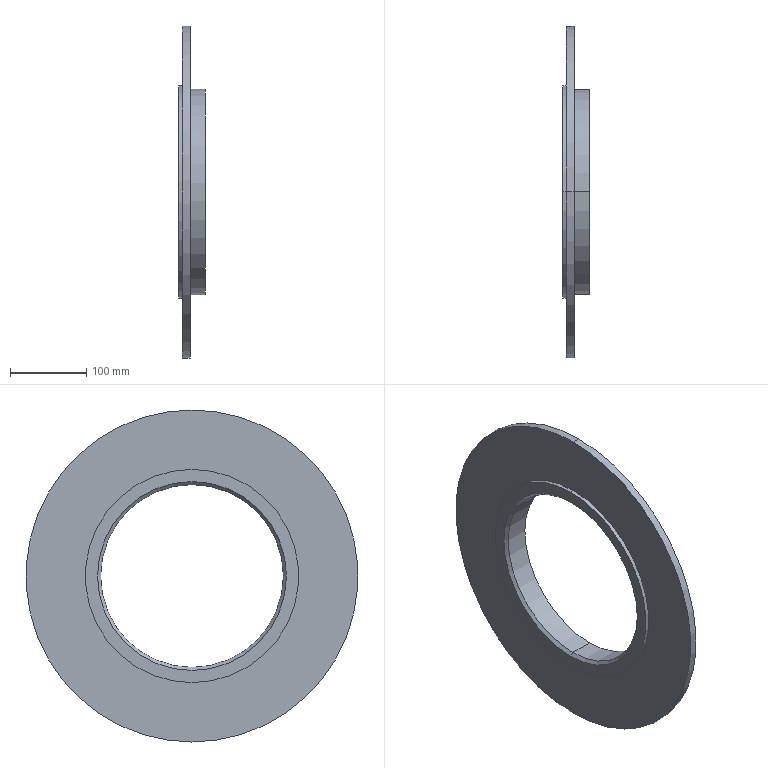Part | SolidWorks | features Chamfer 1, Revolution 1 | 1 solid | 14 faces | box 35 x 436 x 436 mm | volume 1356536 mm3 | cylinder 8 | plane 4 | cone 2 | commonest cylinder face diameters 240 x2 270 x2 280 x2 436 x2
STEP:
#1=CARTESIAN_POINT('',(4.,0.,-120.));
#2=VERTEX_POINT('',#1);
#3=CARTESIAN_POINT('',(4.,0.,120.));
#4=VERTEX_POINT('',#3);
#5=CARTESIAN_POINT('',(4.,0.,0.));
#6=DIRECTION('',(-1.,0.,0.));
#7=DIRECTION('',(0.,0.,-1.));
#8=AXIS2_PLACEMENT_3D('',#5,#6,#7);
#9=CIRCLE('',#8,120.);
#10=EDGE_CURVE('',#2,#4,#9,.T.);
#11=ORIENTED_EDGE('',*,*,#10,.F.);
#12=CARTESIAN_POINT('',(0.,0.,-124.));
#13=VERTEX_POINT('',#12);
#14=CARTESIAN_POINT('',(4.,0.,-120.));
#15=DIRECTION('',(-0.7071,0.,-0.7071));
#16=VECTOR('',#15,1000.);
#17=LINE('',#14,#16);
#18=EDGE_CURVE('',#2,#13,#17,.T.);
#19=ORIENTED_EDGE('',*,*,#18,.T.);
#20=CARTESIAN_POINT('',(0.,0.,124.));
#21=VERTEX_POINT('',#20);
#22=CARTESIAN_POINT('',(0.,0.,0.));
#23=DIRECTION('',(1.,0.,0.));
#24=DIRECTION('',(0.,0.,-1.));
#25=AXIS2_PLACEMENT_3D('',#22,#23,#24);
#26=CIRCLE('',#25,124.);
#27=EDGE_CURVE('',#21,#13,#26,.T.);
#28=ORIENTED_EDGE('',*,*,#27,.F.);
#29=CARTESIAN_POINT('',(4.,0.,120.));
#30=DIRECTION('',(-0.7071,0.,0.7071));
#31=VECTOR('',#30,1000.);
#32=LINE('',#29,#31);
#33=EDGE_CURVE('',#4,#21,#32,.T.);
#34=ORIENTED_EDGE('',*,*,#33,.F.);
#35=EDGE_LOOP('',(#11,#19,#28,#34));
#36=FACE_OUTER_BOUND('',#35,.T.);
#37=CARTESIAN_POINT('',(4.,0.,0.));
#38=DIRECTION('',(-1.,0.,0.));
#39=DIRECTION('',(0.,0.,1.));
#40=AXIS2_PLACEMENT_3D('',#37,#38,#39);
#41=CONICAL_SURFACE('',#40,120.,0.7854);
#42=ADVANCED_FACE('',(#36),#41,.F.);
#43=CARTESIAN_POINT('',(35.,0.,-120.));
#44=VERTEX_POINT('',#43);
#45=CARTESIAN_POINT('',(35.,0.,120.));
#46=VERTEX_POINT('',#45);
#47=CARTESIAN_POINT('',(35.,0.,0.));
#48=DIRECTION('',(-1.,0.,0.));
#49=DIRECTION('',(0.,0.,1.));
#50=AXIS2_PLACEMENT_3D('',#47,#48,#49);
#51=CIRCLE('',#50,120.);
#52=EDGE_CURVE('',#44,#46,#51,.T.);
#53=ORIENTED_EDGE('',*,*,#52,.F.);
#54=CARTESIAN_POINT('',(0.,0.,-120.));
#55=DIRECTION('',(-1.,0.,0.));
#56=VECTOR('',#55,1000.);
#57=LINE('',#54,#56);
#58=EDGE_CURVE('',#44,#2,#57,.T.);
#59=ORIENTED_EDGE('',*,*,#58,.T.);
#60=ORIENTED_EDGE('',*,*,#10,.T.);
#61=CARTESIAN_POINT('',(0.,0.,120.));
#62=DIRECTION('',(-1.,0.,0.));
#63=VECTOR('',#62,1000.);
#64=LINE('',#61,#63);
#65=EDGE_CURVE('',#46,#4,#64,.T.);
#66=ORIENTED_EDGE('',*,*,#65,.F.);
#67=EDGE_LOOP('',(#53,#59,#60,#66));
#68=FACE_OUTER_BOUND('',#67,.T.);
#69=CARTESIAN_POINT('',(0.,0.,0.));
#70=DIRECTION('',(-1.,0.,0.));
#71=DIRECTION('',(0.,0.,1.));
#72=AXIS2_PLACEMENT_3D('',#69,#70,#71);
#73=CYLINDRICAL_SURFACE('',#72,120.);
#74=ADVANCED_FACE('',(#68),#73,.F.);
#75=CARTESIAN_POINT('',(35.,0.,135.));
#76=VERTEX_POINT('',#75);
#77=CARTESIAN_POINT('',(35.,0.,-135.));
#78=VERTEX_POINT('',#77);
#79=CARTESIAN_POINT('',(35.,0.,0.));
#80=DIRECTION('',(-1.,0.,0.));
#81=DIRECTION('',(0.,0.,1.));
#82=AXIS2_PLACEMENT_3D('',#79,#80,#81);
#83=CIRCLE('',#82,135.);
#84=EDGE_CURVE('',#76,#78,#83,.T.);
#85=ORIENTED_EDGE('',*,*,#84,.T.);
#86=CARTESIAN_POINT('',(15.,0.,-135.));
#87=VERTEX_POINT('',#86);
#88=CARTESIAN_POINT('',(0.,0.,-135.));
#89=DIRECTION('',(-1.,0.,0.));
#90=VECTOR('',#89,1000.);
#91=LINE('',#88,#90);
#92=EDGE_CURVE('',#78,#87,#91,.T.);
#93=ORIENTED_EDGE('',*,*,#92,.T.);
#94=CARTESIAN_POINT('',(15.,0.,135.));
#95=VERTEX_POINT('',#94);
#96=CARTESIAN_POINT('',(15.,0.,0.));
#97=DIRECTION('',(-1.,0.,0.));
#98=DIRECTION('',(0.,0.,1.));
#99=AXIS2_PLACEMENT_3D('',#96,#97,#98);
#100=CIRCLE('',#99,135.);
#101=EDGE_CURVE('',#95,#87,#100,.T.);
#102=ORIENTED_EDGE('',*,*,#101,.F.);
#103=CARTESIAN_POINT('',(0.,0.,135.));
#104=DIRECTION('',(-1.,0.,0.));
#105=VECTOR('',#104,1000.);
#106=LINE('',#103,#105);
#107=EDGE_CURVE('',#76,#95,#106,.T.);
#108=ORIENTED_EDGE('',*,*,#107,.F.);
#109=EDGE_LOOP('',(#85,#93,#102,#108));
#110=FACE_OUTER_BOUND('',#109,.T.);
#111=CARTESIAN_POINT('',(0.,0.,0.));
#112=DIRECTION('',(-1.,0.,0.));
#113=DIRECTION('',(0.,0.,1.));
#114=AXIS2_PLACEMENT_3D('',#111,#112,#113);
#115=CYLINDRICAL_SURFACE('',#114,135.);
#116=ADVANCED_FACE('',(#110),#115,.T.);
#117=CARTESIAN_POINT('',(15.,0.,218.));
#118=VERTEX_POINT('',#117);
#119=CARTESIAN_POINT('',(15.,0.,-218.));
#120=VERTEX_POINT('',#119);
#121=CARTESIAN_POINT('',(15.,0.,0.));
#122=DIRECTION('',(-1.,0.,0.));
#123=DIRECTION('',(0.,0.,1.));
#124=AXIS2_PLACEMENT_3D('',#121,#122,#123);
#125=CIRCLE('',#124,218.);
#126=EDGE_CURVE('',#118,#120,#125,.T.);
#127=ORIENTED_EDGE('',*,*,#126,.T.);
#128=CARTESIAN_POINT('',(5.,0.,-218.));
#129=VERTEX_POINT('',#128);
#130=CARTESIAN_POINT('',(0.,0.,-218.));
#131=DIRECTION('',(-1.,0.,0.));
#132=VECTOR('',#131,1000.);
#133=LINE('',#130,#132);
#134=EDGE_CURVE('',#120,#129,#133,.T.);
#135=ORIENTED_EDGE('',*,*,#134,.T.);
#136=CARTESIAN_POINT('',(5.,0.,218.));
#137=VERTEX_POINT('',#136);
#138=CARTESIAN_POINT('',(5.,0.,0.));
#139=DIRECTION('',(-1.,0.,0.));
#140=DIRECTION('',(0.,0.,1.));
#141=AXIS2_PLACEMENT_3D('',#138,#139,#140);
#142=CIRCLE('',#141,218.);
#143=EDGE_CURVE('',#137,#129,#142,.T.);
#144=ORIENTED_EDGE('',*,*,#143,.F.);
#145=CARTESIAN_POINT('',(0.,0.,218.));
#146=DIRECTION('',(-1.,0.,0.));
#147=VECTOR('',#146,1000.);
#148=LINE('',#145,#147);
#149=EDGE_CURVE('',#118,#137,#148,.T.);
#150=ORIENTED_EDGE('',*,*,#149,.F.);
#151=EDGE_LOOP('',(#127,#135,#144,#150));
#152=FACE_OUTER_BOUND('',#151,.T.);
#153=CARTESIAN_POINT('',(0.,0.,0.));
#154=DIRECTION('',(-1.,0.,0.));
#155=DIRECTION('',(0.,0.,1.));
#156=AXIS2_PLACEMENT_3D('',#153,#154,#155);
#157=CYLINDRICAL_SURFACE('',#156,218.);
#158=ADVANCED_FACE('',(#152),#157,.T.);
#159=CARTESIAN_POINT('',(5.,0.,140.));
#160=VERTEX_POINT('',#159);
#161=CARTESIAN_POINT('',(5.,0.,-140.));
#162=VERTEX_POINT('',#161);
#163=CARTESIAN_POINT('',(5.,0.,0.));
#164=DIRECTION('',(-1.,0.,0.));
#165=DIRECTION('',(0.,0.,1.));
#166=AXIS2_PLACEMENT_3D('',#163,#164,#165);
#167=CIRCLE('',#166,140.);
#168=EDGE_CURVE('',#160,#162,#167,.T.);
#169=ORIENTED_EDGE('',*,*,#168,.T.);
#170=CARTESIAN_POINT('',(0.,0.,-140.));
#171=VERTEX_POINT('',#170);
#172=CARTESIAN_POINT('',(0.,0.,-140.));
#173=DIRECTION('',(-1.,0.,0.));
#174=VECTOR('',#173,1000.);
#175=LINE('',#172,#174);
#176=EDGE_CURVE('',#162,#171,#175,.T.);
#177=ORIENTED_EDGE('',*,*,#176,.T.);
#178=CARTESIAN_POINT('',(0.,0.,140.));
#179=VERTEX_POINT('',#178);
#180=CARTESIAN_POINT('',(0.,0.,0.));
#181=DIRECTION('',(-1.,0.,0.));
#182=DIRECTION('',(0.,0.,1.));
#183=AXIS2_PLACEMENT_3D('',#180,#181,#182);
#184=CIRCLE('',#183,140.);
#185=EDGE_CURVE('',#179,#171,#184,.T.);
#186=ORIENTED_EDGE('',*,*,#185,.F.);
#187=CARTESIAN_POINT('',(0.,0.,140.));
#188=DIRECTION('',(-1.,0.,0.));
#189=VECTOR('',#188,1000.);
#190=LINE('',#187,#189);
#191=EDGE_CURVE('',#160,#179,#190,.T.);
#192=ORIENTED_EDGE('',*,*,#191,.F.);
#193=EDGE_LOOP('',(#169,#177,#186,#192));
#194=FACE_OUTER_BOUND('',#193,.T.);
#195=CARTESIAN_POINT('',(0.,0.,0.));
#196=DIRECTION('',(-1.,0.,0.));
#197=DIRECTION('',(0.,0.,1.));
#198=AXIS2_PLACEMENT_3D('',#195,#196,#197);
#199=CYLINDRICAL_SURFACE('',#198,140.);
#200=ADVANCED_FACE('',(#194),#199,.T.);
#201=ORIENTED_EDGE('',*,*,#27,.T.);
#202=CARTESIAN_POINT('',(0.,0.,0.));
#203=DIRECTION('',(1.,0.,0.));
#204=DIRECTION('',(0.,0.,-1.));
#205=AXIS2_PLACEMENT_3D('',#202,#203,#204);
#206=CIRCLE('',#205,124.);
#207=EDGE_CURVE('',#13,#21,#206,.T.);
#208=ORIENTED_EDGE('',*,*,#207,.T.);
#209=EDGE_LOOP('',(#201,#208));
#210=FACE_BOUND('',#209,.T.);
#211=ORIENTED_EDGE('',*,*,#185,.T.);
#212=CARTESIAN_POINT('',(0.,0.,0.));
#213=DIRECTION('',(-1.,0.,0.));
#214=DIRECTION('',(0.,0.,1.));
#215=AXIS2_PLACEMENT_3D('',#212,#213,#214);
#216=CIRCLE('',#215,140.);
#217=EDGE_CURVE('',#171,#179,#216,.T.);
#218=ORIENTED_EDGE('',*,*,#217,.T.);
#219=EDGE_LOOP('',(#211,#218));
#220=FACE_OUTER_BOUND('',#219,.T.);
#221=CARTESIAN_POINT('',(0.,120.,0.));
#222=DIRECTION('',(1.,0.,0.));
#223=DIRECTION('',(0.,0.,-1.));
#224=AXIS2_PLACEMENT_3D('',#221,#222,#223);
#225=PLANE('',#224);
#226=ADVANCED_FACE('',(#210,#220),#225,.F.);
#227=ORIENTED_EDGE('',*,*,#176,.F.);
#228=CARTESIAN_POINT('',(5.,0.,0.));
#229=DIRECTION('',(-1.,0.,0.));
#230=DIRECTION('',(0.,0.,1.));
#231=AXIS2_PLACEMENT_3D('',#228,#229,#230);
#232=CIRCLE('',#231,140.);
#233=EDGE_CURVE('',#162,#160,#232,.T.);
#234=ORIENTED_EDGE('',*,*,#233,.T.);
#235=ORIENTED_EDGE('',*,*,#191,.T.);
#236=ORIENTED_EDGE('',*,*,#217,.F.);
#237=EDGE_LOOP('',(#227,#234,#235,#236));
#238=FACE_OUTER_BOUND('',#237,.T.);
#239=CARTESIAN_POINT('',(0.,0.,0.));
#240=DIRECTION('',(-1.,0.,0.));
#241=DIRECTION('',(0.,0.,1.));
#242=AXIS2_PLACEMENT_3D('',#239,#240,#241);
#243=CYLINDRICAL_SURFACE('',#242,140.);
#244=ADVANCED_FACE('',(#238),#243,.T.);
#245=ORIENTED_EDGE('',*,*,#168,.F.);
#246=ORIENTED_EDGE('',*,*,#233,.F.);
#247=EDGE_LOOP('',(#245,#246));
#248=FACE_BOUND('',#247,.T.);
#249=ORIENTED_EDGE('',*,*,#143,.T.);
#250=CARTESIAN_POINT('',(5.,0.,0.));
#251=DIRECTION('',(-1.,0.,0.));
#252=DIRECTION('',(0.,0.,1.));
#253=AXIS2_PLACEMENT_3D('',#250,#251,#252);
#254=CIRCLE('',#253,218.);
#255=EDGE_CURVE('',#129,#137,#254,.T.);
#256=ORIENTED_EDGE('',*,*,#255,.T.);
#257=EDGE_LOOP('',(#249,#256));
#258=FACE_OUTER_BOUND('',#257,.T.);
#259=CARTESIAN_POINT('',(5.,140.,0.));
#260=DIRECTION('',(1.,0.,0.));
#261=DIRECTION('',(0.,0.,-1.));
#262=AXIS2_PLACEMENT_3D('',#259,#260,#261);
#263=PLANE('',#262);
#264=ADVANCED_FACE('',(#248,#258),#263,.F.);
#265=ORIENTED_EDGE('',*,*,#134,.F.);
#266=CARTESIAN_POINT('',(15.,0.,0.));
#267=DIRECTION('',(-1.,0.,0.));
#268=DIRECTION('',(0.,0.,1.));
#269=AXIS2_PLACEMENT_3D('',#266,#267,#268);
#270=CIRCLE('',#269,218.);
#271=EDGE_CURVE('',#120,#118,#270,.T.);
#272=ORIENTED_EDGE('',*,*,#271,.T.);
#273=ORIENTED_EDGE('',*,*,#149,.T.);
#274=ORIENTED_EDGE('',*,*,#255,.F.);
#275=EDGE_LOOP('',(#265,#272,#273,#274));
#276=FACE_OUTER_BOUND('',#275,.T.);
#277=CARTESIAN_POINT('',(0.,0.,0.));
#278=DIRECTION('',(-1.,0.,0.));
#279=DIRECTION('',(0.,0.,1.));
#280=AXIS2_PLACEMENT_3D('',#277,#278,#279);
#281=CYLINDRICAL_SURFACE('',#280,218.);
#282=ADVANCED_FACE('',(#276),#281,.T.);
#283=ORIENTED_EDGE('',*,*,#126,.F.);
#284=ORIENTED_EDGE('',*,*,#271,.F.);
#285=EDGE_LOOP('',(#283,#284));
#286=FACE_OUTER_BOUND('',#285,.T.);
#287=ORIENTED_EDGE('',*,*,#101,.T.);
#288=CARTESIAN_POINT('',(15.,0.,0.));
#289=DIRECTION('',(-1.,0.,0.));
#290=DIRECTION('',(0.,0.,1.));
#291=AXIS2_PLACEMENT_3D('',#288,#289,#290);
#292=CIRCLE('',#291,135.);
#293=EDGE_CURVE('',#87,#95,#292,.T.);
#294=ORIENTED_EDGE('',*,*,#293,.T.);
#295=EDGE_LOOP('',(#287,#294));
#296=FACE_BOUND('',#295,.T.);
#297=CARTESIAN_POINT('',(15.,218.,0.));
#298=DIRECTION('',(-1.,0.,0.));
#299=DIRECTION('',(0.,0.,1.));
#300=AXIS2_PLACEMENT_3D('',#297,#298,#299);
#301=PLANE('',#300);
#302=ADVANCED_FACE('',(#286,#296),#301,.F.);
#303=ORIENTED_EDGE('',*,*,#92,.F.);
#304=CARTESIAN_POINT('',(35.,0.,0.));
#305=DIRECTION('',(-1.,0.,0.));
#306=DIRECTION('',(0.,0.,1.));
#307=AXIS2_PLACEMENT_3D('',#304,#305,#306);
#308=CIRCLE('',#307,135.);
#309=EDGE_CURVE('',#78,#76,#308,.T.);
#310=ORIENTED_EDGE('',*,*,#309,.T.);
#311=ORIENTED_EDGE('',*,*,#107,.T.);
#312=ORIENTED_EDGE('',*,*,#293,.F.);
#313=EDGE_LOOP('',(#303,#310,#311,#312));
#314=FACE_OUTER_BOUND('',#313,.T.);
#315=CARTESIAN_POINT('',(0.,0.,0.));
#316=DIRECTION('',(-1.,0.,0.));
#317=DIRECTION('',(0.,0.,1.));
#318=AXIS2_PLACEMENT_3D('',#315,#316,#317);
#319=CYLINDRICAL_SURFACE('',#318,135.);
#320=ADVANCED_FACE('',(#314),#319,.T.);
#321=ORIENTED_EDGE('',*,*,#84,.F.);
#322=ORIENTED_EDGE('',*,*,#309,.F.);
#323=EDGE_LOOP('',(#321,#322));
#324=FACE_OUTER_BOUND('',#323,.T.);
#325=CARTESIAN_POINT('',(35.,0.,0.));
#326=DIRECTION('',(-1.,0.,0.));
#327=DIRECTION('',(0.,0.,1.));
#328=AXIS2_PLACEMENT_3D('',#325,#326,#327);
#329=CIRCLE('',#328,120.);
#330=EDGE_CURVE('',#46,#44,#329,.T.);
#331=ORIENTED_EDGE('',*,*,#330,.T.);
#332=ORIENTED_EDGE('',*,*,#52,.T.);
#333=EDGE_LOOP('',(#331,#332));
#334=FACE_BOUND('',#333,.T.);
#335=CARTESIAN_POINT('',(35.,135.,0.));
#336=DIRECTION('',(-1.,0.,0.));
#337=DIRECTION('',(0.,0.,1.));
#338=AXIS2_PLACEMENT_3D('',#335,#336,#337);
#339=PLANE('',#338);
#340=ADVANCED_FACE('',(#324,#334),#339,.F.);
#341=ORIENTED_EDGE('',*,*,#58,.F.);
#342=ORIENTED_EDGE('',*,*,#330,.F.);
#343=ORIENTED_EDGE('',*,*,#65,.T.);
#344=CARTESIAN_POINT('',(4.,0.,0.));
#345=DIRECTION('',(-1.,0.,0.));
#346=DIRECTION('',(0.,0.,-1.));
#347=AXIS2_PLACEMENT_3D('',#344,#345,#346);
#348=CIRCLE('',#347,120.);
#349=EDGE_CURVE('',#4,#2,#348,.T.);
#350=ORIENTED_EDGE('',*,*,#349,.T.);
#351=EDGE_LOOP('',(#341,#342,#343,#350));
#352=FACE_OUTER_BOUND('',#351,.T.);
#353=CARTESIAN_POINT('',(0.,0.,0.));
#354=DIRECTION('',(-1.,0.,0.));
#355=DIRECTION('',(0.,0.,1.));
#356=AXIS2_PLACEMENT_3D('',#353,#354,#355);
#357=CYLINDRICAL_SURFACE('',#356,120.);
#358=ADVANCED_FACE('',(#352),#357,.F.);
#359=ORIENTED_EDGE('',*,*,#18,.F.);
#360=ORIENTED_EDGE('',*,*,#349,.F.);
#361=ORIENTED_EDGE('',*,*,#33,.T.);
#362=ORIENTED_EDGE('',*,*,#207,.F.);
#363=EDGE_LOOP('',(#359,#360,#361,#362));
#364=FACE_OUTER_BOUND('',#363,.T.);
#365=CARTESIAN_POINT('',(4.,0.,0.));
#366=DIRECTION('',(-1.,0.,0.));
#367=DIRECTION('',(0.,0.,1.));
#368=AXIS2_PLACEMENT_3D('',#365,#366,#367);
#369=CONICAL_SURFACE('',#368,120.,0.7854);
#370=ADVANCED_FACE('',(#364),#369,.F.);
#371=CLOSED_SHELL('',(#42,#74,#116,#158,#200,#226,#244,#264,#282,#302,#320,#340,#358,#370));
#372=MANIFOLD_SOLID_BREP('',#371);
#373=CARTESIAN_POINT('',(0.,0.,0.));
#374=DIRECTION('',(0.,0.,1.));
#375=DIRECTION('',(1.,0.,0.));
#376=AXIS2_PLACEMENT_3D('',#373,#374,#375);
#377=(LENGTH_UNIT()NAMED_UNIT(*)SI_UNIT(.MILLI.,.METRE.));
#378=UNCERTAINTY_MEASURE_WITH_UNIT(LENGTH_MEASURE(0.00001),#377,'','');
#379=(NAMED_UNIT(*)PLANE_ANGLE_UNIT()SI_UNIT($,.RADIAN.));
#380=(NAMED_UNIT(*)SI_UNIT($,.STERADIAN.)SOLID_ANGLE_UNIT());
#381=(GEOMETRIC_REPRESENTATION_CONTEXT(3)GLOBAL_UNCERTAINTY_ASSIGNED_CONTEXT((#378))GLOBAL_UNIT_ASSIGNED_CONTEXT((#377,#379,#380))REPRESENTATION_CONTEXT('',''));
#382=ADVANCED_BREP_SHAPE_REPRESENTATION('',(#372,#376),#381);